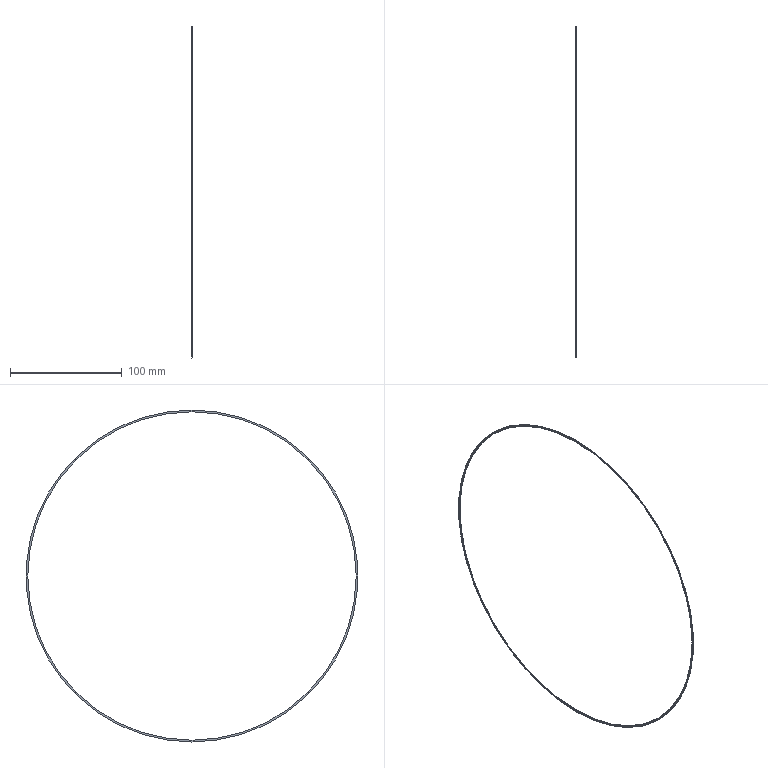Part | SolidWorks | features Revolution 1 | 1 solid | 10 faces | box 0.4 x 296.6 x 296.6 mm | volume 561.725 mm3 | cylinder 4 | torus 2 | cone 2 | plane 2 | commonest cylinder face diameters 293.4 x2 296.6 x2